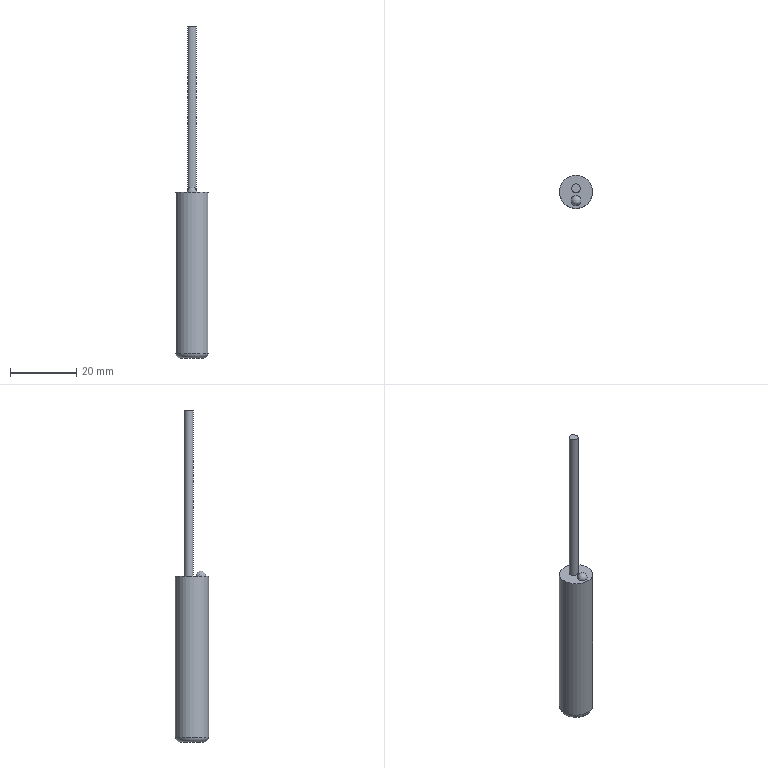Part | STEP file | 冲床-300配套压波_id714_x_t | 1 solid | 7 faces | box 10 x 10 x 100 mm | volume 4206 mm3 | plane 3 | cylinder 2 | sphere 1 | torus 1 | commonest cylinder face diameters 2.7 x1 10 x1
STEP:
#1=CARTESIAN_POINT('',(1540.,-4.15,200.06));
#2=VERTEX_POINT('',#1);
#3=CARTESIAN_POINT('',(1540.,-2.65,200.06));
#4=DIRECTION('',(0.,0.,1.));
#5=DIRECTION('',(0.,-1.,0.));
#6=AXIS2_PLACEMENT_3D('',#3,#4,#5);
#7=CIRCLE('',#6,1.5);
#8=EDGE_CURVE('',#2,#2,#7,.T.);
#9=ORIENTED_EDGE('',*,*,#8,.T.);
#10=EDGE_LOOP('',(#9));
#11=FACE_OUTER_BOUND('',#10,.T.);
#12=CARTESIAN_POINT('',(1540.,-2.65,200.06));
#13=DIRECTION('',(0.,-1.,0.));
#14=DIRECTION('',(0.,0.,1.));
#15=AXIS2_PLACEMENT_3D('',#12,#13,#14);
#16=SPHERICAL_SURFACE('',#15,1.5);
#17=ADVANCED_FACE('',(#11),#16,.T.);
#18=CARTESIAN_POINT('',(1538.65,1.,250.06));
#19=VERTEX_POINT('',#18);
#20=CARTESIAN_POINT('',(1540.,1.,250.06));
#21=DIRECTION('',(0.,0.,-1.));
#22=DIRECTION('',(-1.,0.,0.));
#23=AXIS2_PLACEMENT_3D('',#20,#21,#22);
#24=CIRCLE('',#23,1.35);
#25=EDGE_CURVE('',#19,#19,#24,.T.);
#26=ORIENTED_EDGE('',*,*,#25,.T.);
#27=EDGE_LOOP('',(#26));
#28=FACE_BOUND('',#27,.T.);
#29=CARTESIAN_POINT('',(1538.65,1.,200.06));
#30=VERTEX_POINT('',#29);
#31=CARTESIAN_POINT('',(1540.,1.,200.06));
#32=DIRECTION('',(0.,0.,-1.));
#33=DIRECTION('',(-1.,0.,0.));
#34=AXIS2_PLACEMENT_3D('',#31,#32,#33);
#35=CIRCLE('',#34,1.35);
#36=EDGE_CURVE('',#30,#30,#35,.T.);
#37=ORIENTED_EDGE('',*,*,#36,.F.);
#38=EDGE_LOOP('',(#37));
#39=FACE_BOUND('',#38,.T.);
#40=CARTESIAN_POINT('',(1540.,1.,250.06));
#41=DIRECTION('',(0.,0.,-1.));
#42=DIRECTION('',(0.,1.,0.));
#43=AXIS2_PLACEMENT_3D('',#40,#41,#42);
#44=CYLINDRICAL_SURFACE('',#43,1.35);
#45=ADVANCED_FACE('',(#28,#39),#44,.T.);
#46=ORIENTED_EDGE('',*,*,#25,.F.);
#47=EDGE_LOOP('',(#46));
#48=FACE_OUTER_BOUND('',#47,.T.);
#49=CARTESIAN_POINT('',(1540.,1.,250.06));
#50=DIRECTION('',(0.,0.,-1.));
#51=DIRECTION('',(0.,1.,0.));
#52=AXIS2_PLACEMENT_3D('',#49,#50,#51);
#53=PLANE('',#52);
#54=ADVANCED_FACE('',(#48),#53,.F.);
#55=CARTESIAN_POINT('',(1540.,-3.5,150.06));
#56=VERTEX_POINT('',#55);
#57=CARTESIAN_POINT('',(1540.,0.,150.06));
#58=DIRECTION('',(0.,0.,-1.));
#59=DIRECTION('',(0.,-1.,0.));
#60=AXIS2_PLACEMENT_3D('',#57,#58,#59);
#61=CIRCLE('',#60,3.5);
#62=EDGE_CURVE('',#56,#56,#61,.T.);
#63=ORIENTED_EDGE('',*,*,#62,.T.);
#64=EDGE_LOOP('',(#63));
#65=FACE_OUTER_BOUND('',#64,.T.);
#66=CARTESIAN_POINT('',(1540.,0.,150.06));
#67=DIRECTION('',(0.,0.,1.));
#68=DIRECTION('',(0.,-1.,0.));
#69=AXIS2_PLACEMENT_3D('',#66,#67,#68);
#70=PLANE('',#69);
#71=ADVANCED_FACE('',(#65),#70,.F.);
#72=ORIENTED_EDGE('',*,*,#8,.F.);
#73=EDGE_LOOP('',(#72));
#74=FACE_BOUND('',#73,.T.);
#75=CARTESIAN_POINT('',(1540.,-5.,200.06));
#76=VERTEX_POINT('',#75);
#77=CARTESIAN_POINT('',(1540.,0.,200.06));
#78=DIRECTION('',(0.,0.,1.));
#79=DIRECTION('',(0.,-1.,0.));
#80=AXIS2_PLACEMENT_3D('',#77,#78,#79);
#81=CIRCLE('',#80,5.);
#82=EDGE_CURVE('',#76,#76,#81,.T.);
#83=ORIENTED_EDGE('',*,*,#82,.T.);
#84=EDGE_LOOP('',(#83));
#85=FACE_BOUND('',#84,.T.);
#86=ORIENTED_EDGE('',*,*,#36,.T.);
#87=EDGE_LOOP('',(#86));
#88=FACE_BOUND('',#87,.T.);
#89=CARTESIAN_POINT('',(1540.,0.,200.06));
#90=DIRECTION('',(0.,0.,1.));
#91=DIRECTION('',(0.,-1.,0.));
#92=AXIS2_PLACEMENT_3D('',#89,#90,#91);
#93=PLANE('',#92);
#94=ADVANCED_FACE('',(#74,#85,#88),#93,.T.);
#95=CARTESIAN_POINT('',(1540.,-5.,151.56));
#96=VERTEX_POINT('',#95);
#97=CARTESIAN_POINT('',(1540.,0.,151.56));
#98=DIRECTION('',(0.,0.,1.));
#99=DIRECTION('',(0.,-1.,0.));
#100=AXIS2_PLACEMENT_3D('',#97,#98,#99);
#101=CIRCLE('',#100,5.);
#102=EDGE_CURVE('',#96,#96,#101,.T.);
#103=ORIENTED_EDGE('',*,*,#102,.T.);
#104=EDGE_LOOP('',(#103));
#105=FACE_BOUND('',#104,.T.);
#106=ORIENTED_EDGE('',*,*,#82,.F.);
#107=EDGE_LOOP('',(#106));
#108=FACE_BOUND('',#107,.T.);
#109=CARTESIAN_POINT('',(1540.,0.,180.06));
#110=DIRECTION('',(0.,0.,-1.));
#111=DIRECTION('',(0.,1.,0.));
#112=AXIS2_PLACEMENT_3D('',#109,#110,#111);
#113=CYLINDRICAL_SURFACE('',#112,5.);
#114=ADVANCED_FACE('',(#105,#108),#113,.T.);
#115=ORIENTED_EDGE('',*,*,#62,.F.);
#116=EDGE_LOOP('',(#115));
#117=FACE_BOUND('',#116,.T.);
#118=ORIENTED_EDGE('',*,*,#102,.F.);
#119=EDGE_LOOP('',(#118));
#120=FACE_BOUND('',#119,.T.);
#121=CARTESIAN_POINT('',(1540.,0.,151.56));
#122=DIRECTION('',(0.,0.,1.));
#123=DIRECTION('',(0.,-1.,0.));
#124=AXIS2_PLACEMENT_3D('',#121,#122,#123);
#125=TOROIDAL_SURFACE('',#124,3.5,1.5);
#126=ADVANCED_FACE('',(#117,#120),#125,.T.);
#127=CLOSED_SHELL('',(#17,#45,#54,#71,#94,#114,#126));
#128=MANIFOLD_SOLID_BREP('',#127);
#129=(LENGTH_UNIT()NAMED_UNIT(*)SI_UNIT(.MILLI.,.METRE.));
#130=UNCERTAINTY_MEASURE_WITH_UNIT(LENGTH_MEASURE(0.00002),#129,'','');
#131=(NAMED_UNIT(*)PLANE_ANGLE_UNIT()SI_UNIT($,.RADIAN.));
#132=PLANE_ANGLE_MEASURE_WITH_UNIT(PLANE_ANGLE_MEASURE(0.01745),#131);
#133=DIMENSIONAL_EXPONENTS(0.,0.,0.,0.,0.,0.,0.);
#134=(CONVERSION_BASED_UNIT('DEGREE',#132)NAMED_UNIT(#133)PLANE_ANGLE_UNIT());
#135=(NAMED_UNIT(*)SI_UNIT($,.STERADIAN.)SOLID_ANGLE_UNIT());
#136=(GEOMETRIC_REPRESENTATION_CONTEXT(3)GLOBAL_UNCERTAINTY_ASSIGNED_CONTEXT((#130))GLOBAL_UNIT_ASSIGNED_CONTEXT((#129,#134,#135))REPRESENTATION_CONTEXT('',''));
#137=ADVANCED_BREP_SHAPE_REPRESENTATION('',(#128),#136);